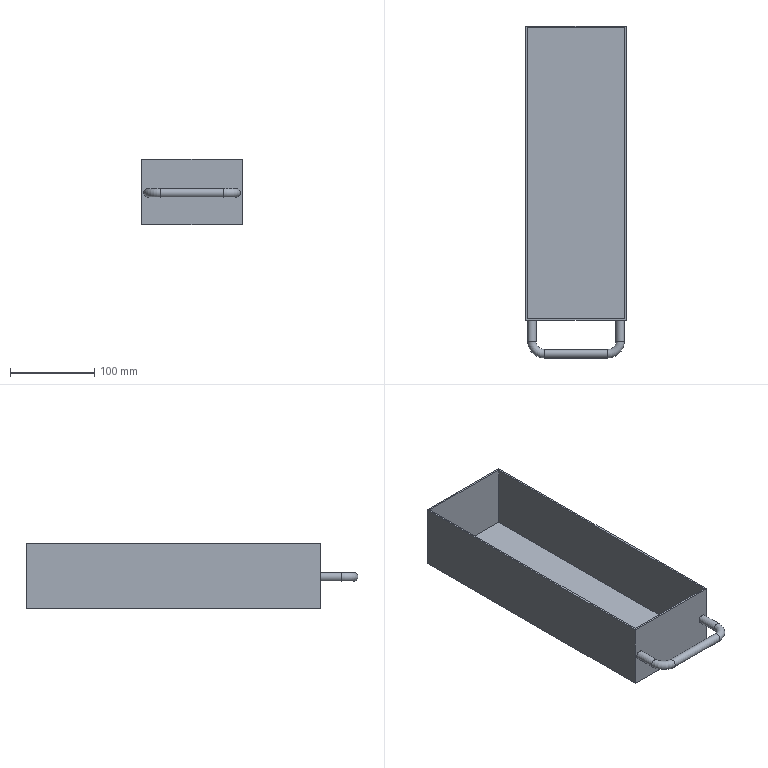Part | NX | features solid 2 | 1 solid | 16 faces | box 120 x 395 x 78 mm | volume 239183 mm3 | plane 11 | cylinder 3 | torus 2 | commonest cylinder face diameters 10 x3
STEP:
#1=CARTESIAN_POINT('',(-715.,-405.,-320.));
#2=VERTEX_POINT('',#1);
#3=CARTESIAN_POINT('',(-595.,-405.,-320.));
#4=VERTEX_POINT('',#3);
#5=CARTESIAN_POINT('',(-1120.,-405.,-320.));
#6=DIRECTION('',(1.,0.,0.));
#7=VECTOR('',#6,1000.);
#8=LINE('',#5,#7);
#9=EDGE_CURVE('',#2,#4,#8,.T.);
#10=ORIENTED_EDGE('',*,*,#9,.T.);
#11=CARTESIAN_POINT('',(-595.,-405.,-242.));
#12=VERTEX_POINT('',#11);
#13=CARTESIAN_POINT('',(-595.,-405.,200.));
#14=DIRECTION('',(0.,0.,1.));
#15=VECTOR('',#14,1000.);
#16=LINE('',#13,#15);
#17=EDGE_CURVE('',#12,#4,#16,.F.);
#18=ORIENTED_EDGE('',*,*,#17,.F.);
#19=CARTESIAN_POINT('',(-715.,-405.,-242.));
#20=VERTEX_POINT('',#19);
#21=CARTESIAN_POINT('',(-1120.,-405.,-242.));
#22=DIRECTION('',(-1.,0.,0.));
#23=VECTOR('',#22,1000.);
#24=LINE('',#21,#23);
#25=EDGE_CURVE('',#20,#12,#24,.F.);
#26=ORIENTED_EDGE('',*,*,#25,.F.);
#27=CARTESIAN_POINT('',(-715.,-405.,-85.));
#28=DIRECTION('',(0.,0.,1.));
#29=VECTOR('',#28,1000.);
#30=LINE('',#27,#29);
#31=EDGE_CURVE('',#20,#2,#30,.F.);
#32=ORIENTED_EDGE('',*,*,#31,.T.);
#33=EDGE_LOOP('',(#10,#18,#26,#32));
#34=FACE_BOUND('',#33,.T.);
#35=CARTESIAN_POINT('',(-702.5,-405.,-282.));
#36=VERTEX_POINT('',#35);
#37=CARTESIAN_POINT('',(-707.5,-405.,-282.));
#38=DIRECTION('',(0.,1.,0.));
#39=DIRECTION('',(1.,0.,0.));
#40=AXIS2_PLACEMENT_3D('',#37,#38,#39);
#41=CIRCLE('',#40,5.);
#42=EDGE_CURVE('',#36,#36,#41,.T.);
#43=ORIENTED_EDGE('',*,*,#42,.T.);
#44=EDGE_LOOP('',(#43));
#45=FACE_BOUND('',#44,.T.);
#46=CARTESIAN_POINT('',(-602.5,-405.,-287.));
#47=VERTEX_POINT('',#46);
#48=CARTESIAN_POINT('',(-602.5,-405.,-282.));
#49=DIRECTION('',(0.,-1.,0.));
#50=DIRECTION('',(0.,0.,-1.));
#51=AXIS2_PLACEMENT_3D('',#48,#49,#50);
#52=CIRCLE('',#51,5.);
#53=EDGE_CURVE('',#47,#47,#52,.T.);
#54=ORIENTED_EDGE('',*,*,#53,.F.);
#55=EDGE_LOOP('',(#54));
#56=FACE_BOUND('',#55,.T.);
#57=CARTESIAN_POINT('',(-1120.,-405.,-85.));
#58=DIRECTION('',(0.,-1.,0.));
#59=DIRECTION('',(0.,0.,-1.));
#60=AXIS2_PLACEMENT_3D('',#57,#58,#59);
#61=PLANE('',#60);
#62=ADVANCED_FACE('',(#34,#45,#56),#61,.T.);
#63=CARTESIAN_POINT('',(-595.,-55.,-320.));
#64=VERTEX_POINT('',#63);
#65=CARTESIAN_POINT('',(-595.,-15.,-320.));
#66=DIRECTION('',(0.,-1.,0.));
#67=VECTOR('',#66,1000.);
#68=LINE('',#65,#67);
#69=EDGE_CURVE('',#4,#64,#68,.F.);
#70=ORIENTED_EDGE('',*,*,#69,.T.);
#71=CARTESIAN_POINT('',(-595.,-55.,-242.));
#72=VERTEX_POINT('',#71);
#73=CARTESIAN_POINT('',(-595.,-55.,-175.));
#74=DIRECTION('',(0.,0.,1.));
#75=VECTOR('',#74,1000.);
#76=LINE('',#73,#75);
#77=EDGE_CURVE('',#72,#64,#76,.F.);
#78=ORIENTED_EDGE('',*,*,#77,.F.);
#79=CARTESIAN_POINT('',(-595.,-15.,-242.));
#80=DIRECTION('',(0.,1.,0.));
#81=VECTOR('',#80,1000.);
#82=LINE('',#79,#81);
#83=EDGE_CURVE('',#12,#72,#82,.T.);
#84=ORIENTED_EDGE('',*,*,#83,.F.);
#85=ORIENTED_EDGE('',*,*,#17,.T.);
#86=EDGE_LOOP('',(#70,#78,#84,#85));
#87=FACE_BOUND('',#86,.T.);
#88=CARTESIAN_POINT('',(-595.,-15.,200.));
#89=DIRECTION('',(-1.,0.,0.));
#90=DIRECTION('',(0.,0.,1.));
#91=AXIS2_PLACEMENT_3D('',#88,#89,#90);
#92=PLANE('',#91);
#93=ADVANCED_FACE('',(#87),#92,.F.);
#94=CARTESIAN_POINT('',(-715.,-55.,-320.));
#95=VERTEX_POINT('',#94);
#96=CARTESIAN_POINT('',(-590.,-55.,-320.));
#97=DIRECTION('',(-1.,0.,0.));
#98=VECTOR('',#97,1000.);
#99=LINE('',#96,#98);
#100=EDGE_CURVE('',#64,#95,#99,.T.);
#101=ORIENTED_EDGE('',*,*,#100,.T.);
#102=CARTESIAN_POINT('',(-715.,-55.,-242.));
#103=VERTEX_POINT('',#102);
#104=CARTESIAN_POINT('',(-715.,-55.,200.));
#105=DIRECTION('',(0.,0.,1.));
#106=VECTOR('',#105,1000.);
#107=LINE('',#104,#106);
#108=EDGE_CURVE('',#103,#95,#107,.F.);
#109=ORIENTED_EDGE('',*,*,#108,.F.);
#110=CARTESIAN_POINT('',(-590.,-55.,-242.));
#111=DIRECTION('',(1.,0.,0.));
#112=VECTOR('',#111,1000.);
#113=LINE('',#110,#112);
#114=EDGE_CURVE('',#72,#103,#113,.F.);
#115=ORIENTED_EDGE('',*,*,#114,.F.);
#116=ORIENTED_EDGE('',*,*,#77,.T.);
#117=EDGE_LOOP('',(#101,#109,#115,#116));
#118=FACE_BOUND('',#117,.T.);
#119=CARTESIAN_POINT('',(-590.,-55.,-175.));
#120=DIRECTION('',(0.,1.,0.));
#121=DIRECTION('',(-1.,0.,0.));
#122=AXIS2_PLACEMENT_3D('',#119,#120,#121);
#123=PLANE('',#122);
#124=ADVANCED_FACE('',(#118),#123,.T.);
#125=CARTESIAN_POINT('',(-715.,580.,-320.));
#126=DIRECTION('',(0.,1.,0.));
#127=VECTOR('',#126,1000.);
#128=LINE('',#125,#127);
#129=EDGE_CURVE('',#95,#2,#128,.F.);
#130=ORIENTED_EDGE('',*,*,#129,.T.);
#131=ORIENTED_EDGE('',*,*,#31,.F.);
#132=CARTESIAN_POINT('',(-715.,580.,-242.));
#133=DIRECTION('',(0.,-1.,0.));
#134=VECTOR('',#133,1000.);
#135=LINE('',#132,#134);
#136=EDGE_CURVE('',#103,#20,#135,.T.);
#137=ORIENTED_EDGE('',*,*,#136,.F.);
#138=ORIENTED_EDGE('',*,*,#108,.T.);
#139=EDGE_LOOP('',(#130,#131,#137,#138));
#140=FACE_BOUND('',#139,.T.);
#141=CARTESIAN_POINT('',(-715.,580.,200.));
#142=DIRECTION('',(1.,0.,0.));
#143=DIRECTION('',(0.,0.,-1.));
#144=AXIS2_PLACEMENT_3D('',#141,#142,#143);
#145=PLANE('',#144);
#146=ADVANCED_FACE('',(#140),#145,.F.);
#147=CARTESIAN_POINT('',(-597.,-403.,-242.));
#148=VERTEX_POINT('',#147);
#149=CARTESIAN_POINT('',(-597.,-57.,-242.));
#150=VERTEX_POINT('',#149);
#151=CARTESIAN_POINT('',(-597.,-15.,-242.));
#152=DIRECTION('',(0.,1.,0.));
#153=VECTOR('',#152,1000.);
#154=LINE('',#151,#153);
#155=EDGE_CURVE('',#148,#150,#154,.T.);
#156=ORIENTED_EDGE('',*,*,#155,.F.);
#157=CARTESIAN_POINT('',(-713.,-403.,-242.));
#158=VERTEX_POINT('',#157);
#159=CARTESIAN_POINT('',(-1120.,-403.,-242.));
#160=DIRECTION('',(-1.,0.,0.));
#161=VECTOR('',#160,1000.);
#162=LINE('',#159,#161);
#163=EDGE_CURVE('',#158,#148,#162,.F.);
#164=ORIENTED_EDGE('',*,*,#163,.F.);
#165=CARTESIAN_POINT('',(-713.,-57.,-242.));
#166=VERTEX_POINT('',#165);
#167=CARTESIAN_POINT('',(-713.,580.,-242.));
#168=DIRECTION('',(0.,-1.,0.));
#169=VECTOR('',#168,1000.);
#170=LINE('',#167,#169);
#171=EDGE_CURVE('',#166,#158,#170,.T.);
#172=ORIENTED_EDGE('',*,*,#171,.F.);
#173=CARTESIAN_POINT('',(-590.,-57.,-242.));
#174=DIRECTION('',(1.,0.,0.));
#175=VECTOR('',#174,1000.);
#176=LINE('',#173,#175);
#177=EDGE_CURVE('',#150,#166,#176,.F.);
#178=ORIENTED_EDGE('',*,*,#177,.F.);
#179=EDGE_LOOP('',(#156,#164,#172,#178));
#180=FACE_BOUND('',#179,.T.);
#181=ORIENTED_EDGE('',*,*,#83,.T.);
#182=ORIENTED_EDGE('',*,*,#114,.T.);
#183=ORIENTED_EDGE('',*,*,#136,.T.);
#184=ORIENTED_EDGE('',*,*,#25,.T.);
#185=EDGE_LOOP('',(#181,#182,#183,#184));
#186=FACE_BOUND('',#185,.T.);
#187=CARTESIAN_POINT('',(-595.,580.,-242.));
#188=DIRECTION('',(0.,0.,1.));
#189=DIRECTION('',(1.,0.,0.));
#190=AXIS2_PLACEMENT_3D('',#187,#188,#189);
#191=PLANE('',#190);
#192=ADVANCED_FACE('',(#180,#186),#191,.T.);
#193=ORIENTED_EDGE('',*,*,#69,.F.);
#194=ORIENTED_EDGE('',*,*,#9,.F.);
#195=ORIENTED_EDGE('',*,*,#129,.F.);
#196=ORIENTED_EDGE('',*,*,#100,.F.);
#197=EDGE_LOOP('',(#193,#194,#195,#196));
#198=FACE_BOUND('',#197,.T.);
#199=CARTESIAN_POINT('',(-560.,-70.,-320.));
#200=DIRECTION('',(0.,0.,-1.));
#201=DIRECTION('',(-1.,0.,0.));
#202=AXIS2_PLACEMENT_3D('',#199,#200,#201);
#203=PLANE('',#202);
#204=ADVANCED_FACE('',(#198),#203,.T.);
#205=CARTESIAN_POINT('',(-597.,-403.,-318.));
#206=VERTEX_POINT('',#205);
#207=CARTESIAN_POINT('',(-597.,-57.,-318.));
#208=VERTEX_POINT('',#207);
#209=CARTESIAN_POINT('',(-597.,-15.,-318.));
#210=DIRECTION('',(0.,-1.,0.));
#211=VECTOR('',#210,1000.);
#212=LINE('',#209,#211);
#213=EDGE_CURVE('',#206,#208,#212,.F.);
#214=ORIENTED_EDGE('',*,*,#213,.F.);
#215=CARTESIAN_POINT('',(-597.,-403.,200.));
#216=DIRECTION('',(0.,0.,1.));
#217=VECTOR('',#216,1000.);
#218=LINE('',#215,#217);
#219=EDGE_CURVE('',#148,#206,#218,.F.);
#220=ORIENTED_EDGE('',*,*,#219,.F.);
#221=ORIENTED_EDGE('',*,*,#155,.T.);
#222=CARTESIAN_POINT('',(-597.,-57.,-175.));
#223=DIRECTION('',(0.,0.,1.));
#224=VECTOR('',#223,1000.);
#225=LINE('',#222,#224);
#226=EDGE_CURVE('',#150,#208,#225,.F.);
#227=ORIENTED_EDGE('',*,*,#226,.T.);
#228=EDGE_LOOP('',(#214,#220,#221,#227));
#229=FACE_BOUND('',#228,.T.);
#230=CARTESIAN_POINT('',(-597.,-15.,200.));
#231=DIRECTION('',(-1.,0.,0.));
#232=DIRECTION('',(0.,0.,1.));
#233=AXIS2_PLACEMENT_3D('',#230,#231,#232);
#234=PLANE('',#233);
#235=ADVANCED_FACE('',(#229),#234,.T.);
#236=CARTESIAN_POINT('',(-713.,-57.,-318.));
#237=VERTEX_POINT('',#236);
#238=CARTESIAN_POINT('',(-590.,-57.,-318.));
#239=DIRECTION('',(-1.,0.,0.));
#240=VECTOR('',#239,1000.);
#241=LINE('',#238,#240);
#242=EDGE_CURVE('',#208,#237,#241,.T.);
#243=ORIENTED_EDGE('',*,*,#242,.F.);
#244=ORIENTED_EDGE('',*,*,#226,.F.);
#245=ORIENTED_EDGE('',*,*,#177,.T.);
#246=CARTESIAN_POINT('',(-713.,-57.,200.));
#247=DIRECTION('',(0.,0.,1.));
#248=VECTOR('',#247,1000.);
#249=LINE('',#246,#248);
#250=EDGE_CURVE('',#166,#237,#249,.F.);
#251=ORIENTED_EDGE('',*,*,#250,.T.);
#252=EDGE_LOOP('',(#243,#244,#245,#251));
#253=FACE_BOUND('',#252,.T.);
#254=CARTESIAN_POINT('',(-590.,-57.,-175.));
#255=DIRECTION('',(0.,1.,0.));
#256=DIRECTION('',(-1.,0.,0.));
#257=AXIS2_PLACEMENT_3D('',#254,#255,#256);
#258=PLANE('',#257);
#259=ADVANCED_FACE('',(#253),#258,.F.);
#260=CARTESIAN_POINT('',(-713.,-403.,-318.));
#261=VERTEX_POINT('',#260);
#262=CARTESIAN_POINT('',(-713.,580.,-318.));
#263=DIRECTION('',(0.,1.,0.));
#264=VECTOR('',#263,1000.);
#265=LINE('',#262,#264);
#266=EDGE_CURVE('',#237,#261,#265,.F.);
#267=ORIENTED_EDGE('',*,*,#266,.F.);
#268=ORIENTED_EDGE('',*,*,#250,.F.);
#269=ORIENTED_EDGE('',*,*,#171,.T.);
#270=CARTESIAN_POINT('',(-713.,-403.,-85.));
#271=DIRECTION('',(0.,0.,1.));
#272=VECTOR('',#271,1000.);
#273=LINE('',#270,#272);
#274=EDGE_CURVE('',#158,#261,#273,.F.);
#275=ORIENTED_EDGE('',*,*,#274,.T.);
#276=EDGE_LOOP('',(#267,#268,#269,#275));
#277=FACE_BOUND('',#276,.T.);
#278=CARTESIAN_POINT('',(-713.,580.,200.));
#279=DIRECTION('',(1.,0.,0.));
#280=DIRECTION('',(0.,0.,-1.));
#281=AXIS2_PLACEMENT_3D('',#278,#279,#280);
#282=PLANE('',#281);
#283=ADVANCED_FACE('',(#277),#282,.T.);
#284=CARTESIAN_POINT('',(-1120.,-403.,-318.));
#285=DIRECTION('',(1.,0.,0.));
#286=VECTOR('',#285,1000.);
#287=LINE('',#284,#286);
#288=EDGE_CURVE('',#261,#206,#287,.T.);
#289=ORIENTED_EDGE('',*,*,#288,.F.);
#290=ORIENTED_EDGE('',*,*,#274,.F.);
#291=ORIENTED_EDGE('',*,*,#163,.T.);
#292=ORIENTED_EDGE('',*,*,#219,.T.);
#293=EDGE_LOOP('',(#289,#290,#291,#292));
#294=FACE_BOUND('',#293,.T.);
#295=CARTESIAN_POINT('',(-1120.,-403.,-85.));
#296=DIRECTION('',(0.,-1.,0.));
#297=DIRECTION('',(0.,0.,-1.));
#298=AXIS2_PLACEMENT_3D('',#295,#296,#297);
#299=PLANE('',#298);
#300=ADVANCED_FACE('',(#294),#299,.F.);
#301=ORIENTED_EDGE('',*,*,#213,.T.);
#302=ORIENTED_EDGE('',*,*,#242,.T.);
#303=ORIENTED_EDGE('',*,*,#266,.T.);
#304=ORIENTED_EDGE('',*,*,#288,.T.);
#305=EDGE_LOOP('',(#301,#302,#303,#304));
#306=FACE_BOUND('',#305,.T.);
#307=CARTESIAN_POINT('',(-560.,-70.,-318.));
#308=DIRECTION('',(0.,0.,-1.));
#309=DIRECTION('',(-1.,0.,0.));
#310=AXIS2_PLACEMENT_3D('',#307,#308,#309);
#311=PLANE('',#310);
#312=ADVANCED_FACE('',(#306),#311,.F.);
#313=CARTESIAN_POINT('',(-617.5,-440.,-282.));
#314=VERTEX_POINT('',#313);
#315=CARTESIAN_POINT('',(-617.5,-445.,-282.));
#316=DIRECTION('',(-1.,0.,0.));
#317=DIRECTION('',(0.,1.,0.));
#318=AXIS2_PLACEMENT_3D('',#315,#316,#317);
#319=CIRCLE('',#318,5.);
#320=EDGE_CURVE('',#314,#314,#319,.T.);
#321=ORIENTED_EDGE('',*,*,#320,.T.);
#322=EDGE_LOOP('',(#321));
#323=FACE_BOUND('',#322,.T.);
#324=CARTESIAN_POINT('',(-692.5,-440.,-282.));
#325=VERTEX_POINT('',#324);
#326=CARTESIAN_POINT('',(-692.5,-445.,-282.));
#327=DIRECTION('',(-1.,0.,0.));
#328=DIRECTION('',(0.,1.,0.));
#329=AXIS2_PLACEMENT_3D('',#326,#327,#328);
#330=CIRCLE('',#329,5.);
#331=EDGE_CURVE('',#325,#325,#330,.T.);
#332=ORIENTED_EDGE('',*,*,#331,.F.);
#333=EDGE_LOOP('',(#332));
#334=FACE_BOUND('',#333,.T.);
#335=CARTESIAN_POINT('',(-667.5,-445.,-282.));
#336=DIRECTION('',(1.,0.,0.));
#337=DIRECTION('',(0.,0.,-1.));
#338=AXIS2_PLACEMENT_3D('',#335,#336,#337);
#339=CYLINDRICAL_SURFACE('',#338,5.);
#340=ADVANCED_FACE('',(#323,#334),#339,.T.);
#341=CARTESIAN_POINT('',(-702.5,-430.,-282.));
#342=VERTEX_POINT('',#341);
#343=CARTESIAN_POINT('',(-707.5,-430.,-282.));
#344=DIRECTION('',(0.,1.,0.));
#345=DIRECTION('',(1.,0.,0.));
#346=AXIS2_PLACEMENT_3D('',#343,#344,#345);
#347=CIRCLE('',#346,5.);
#348=EDGE_CURVE('',#342,#342,#347,.T.);
#349=ORIENTED_EDGE('',*,*,#348,.F.);
#350=EDGE_LOOP('',(#349));
#351=FACE_BOUND('',#350,.T.);
#352=ORIENTED_EDGE('',*,*,#331,.T.);
#353=EDGE_LOOP('',(#352));
#354=FACE_BOUND('',#353,.T.);
#355=CARTESIAN_POINT('',(-692.5,-430.,-282.));
#356=DIRECTION('',(0.,0.,1.));
#357=DIRECTION('',(1.,0.,0.));
#358=AXIS2_PLACEMENT_3D('',#355,#356,#357);
#359=TOROIDAL_SURFACE('',#358,15.,5.);
#360=ADVANCED_FACE('',(#351,#354),#359,.T.);
#361=ORIENTED_EDGE('',*,*,#348,.T.);
#362=EDGE_LOOP('',(#361));
#363=FACE_BOUND('',#362,.T.);
#364=ORIENTED_EDGE('',*,*,#42,.F.);
#365=EDGE_LOOP('',(#364));
#366=FACE_BOUND('',#365,.T.);
#367=CARTESIAN_POINT('',(-707.5,-430.,-282.));
#368=DIRECTION('',(0.,1.,0.));
#369=DIRECTION('',(0.,0.,1.));
#370=AXIS2_PLACEMENT_3D('',#367,#368,#369);
#371=CYLINDRICAL_SURFACE('',#370,5.);
#372=ADVANCED_FACE('',(#363,#366),#371,.T.);
#373=CARTESIAN_POINT('',(-607.5,-430.,-282.));
#374=VERTEX_POINT('',#373);
#375=CARTESIAN_POINT('',(-602.5,-430.,-282.));
#376=DIRECTION('',(0.,-1.,0.));
#377=DIRECTION('',(-1.,0.,0.));
#378=AXIS2_PLACEMENT_3D('',#375,#376,#377);
#379=CIRCLE('',#378,5.);
#380=EDGE_CURVE('',#374,#374,#379,.T.);
#381=ORIENTED_EDGE('',*,*,#380,.F.);
#382=EDGE_LOOP('',(#381));
#383=FACE_BOUND('',#382,.T.);
#384=ORIENTED_EDGE('',*,*,#53,.T.);
#385=EDGE_LOOP('',(#384));
#386=FACE_BOUND('',#385,.T.);
#387=CARTESIAN_POINT('',(-602.5,-430.,-282.));
#388=DIRECTION('',(0.,1.,0.));
#389=DIRECTION('',(0.,0.,1.));
#390=AXIS2_PLACEMENT_3D('',#387,#388,#389);
#391=CYLINDRICAL_SURFACE('',#390,5.);
#392=ADVANCED_FACE('',(#383,#386),#391,.T.);
#393=ORIENTED_EDGE('',*,*,#320,.F.);
#394=EDGE_LOOP('',(#393));
#395=FACE_BOUND('',#394,.T.);
#396=ORIENTED_EDGE('',*,*,#380,.T.);
#397=EDGE_LOOP('',(#396));
#398=FACE_BOUND('',#397,.T.);
#399=CARTESIAN_POINT('',(-617.5,-430.,-282.));
#400=DIRECTION('',(0.,0.,1.));
#401=DIRECTION('',(1.,0.,0.));
#402=AXIS2_PLACEMENT_3D('',#399,#400,#401);
#403=TOROIDAL_SURFACE('',#402,15.,5.);
#404=ADVANCED_FACE('',(#395,#398),#403,.T.);
#405=CLOSED_SHELL('',(#62,#93,#124,#146,#192,#204,#235,#259,#283,#300,#312,#340,#360,#372,#392,#404));
#406=MANIFOLD_SOLID_BREP('',#405);
#407=(LENGTH_UNIT()NAMED_UNIT(*)SI_UNIT(.MILLI.,.METRE.));
#408=UNCERTAINTY_MEASURE_WITH_UNIT(LENGTH_MEASURE(0.00001),#407,'','');
#409=(NAMED_UNIT(*)PLANE_ANGLE_UNIT()SI_UNIT($,.RADIAN.));
#410=(NAMED_UNIT(*)SI_UNIT($,.STERADIAN.)SOLID_ANGLE_UNIT());
#411=(GEOMETRIC_REPRESENTATION_CONTEXT(3)GLOBAL_UNCERTAINTY_ASSIGNED_CONTEXT((#408))GLOBAL_UNIT_ASSIGNED_CONTEXT((#407,#409,#410))REPRESENTATION_CONTEXT('',''));
#412=ADVANCED_BREP_SHAPE_REPRESENTATION('',(#406),#411);